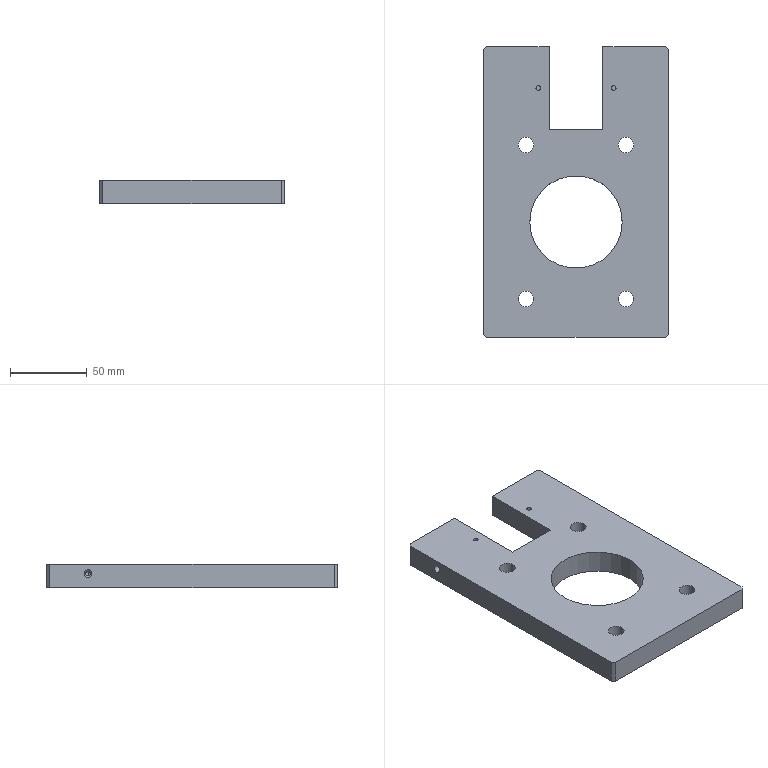Part | SolidWorks | features 3DProfileFeature 6, HoleWzd 6, ICE 2, Extrusion 1 | 3 solids | 60 faces | box 120 x 189 x 15 mm | volume 263341 mm3 | cylinder 34 | plane 18 | cone 8 | commonest cylinder face diameters 3 x20 10.2 x8 5 x4 60 x2